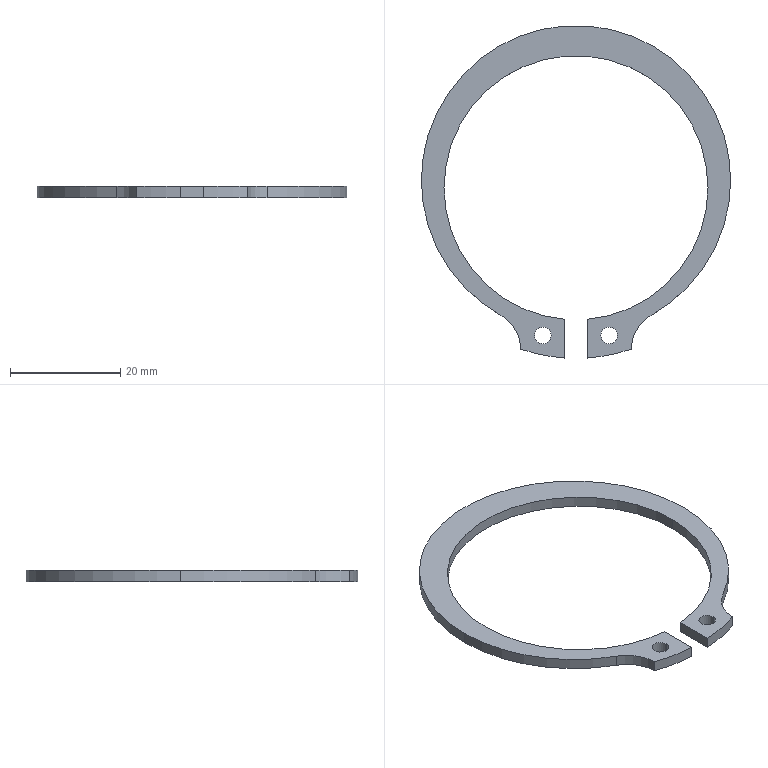Part | STEP file | circlips for shaft--type b gb_GB_CONNECTING_PIECE_RINGS_CSB 52 | 1 solid | 18 faces | box 56 x 60.185 x 2 mm | volume 1438 mm3 | cylinder 14 | plane 4 | commonest cylinder face diameters 3 x4 47.8 x3 56 x3 14 x2 61.76 x2
STEP:
#1=CARTESIAN_POINT('',(0.,0.,0.));
#2=DIRECTION('',(0.,0.,1.));
#3=DIRECTION('',(1.,0.,0.));
#4=AXIS2_PLACEMENT_3D('',#1,#2,#3);
#5=CARTESIAN_POINT('',(7.5,-28.105,-2.));
#6=VERTEX_POINT('',#5);
#7=CARTESIAN_POINT('',(7.5,-28.105,0.));
#8=VERTEX_POINT('',#7);
#9=CARTESIAN_POINT('',(7.5,-28.105,-2.));
#10=DIRECTION('',(0.,0.,1.));
#11=VECTOR('',#10,1.);
#12=LINE('',#9,#11);
#13=CARTESIAN_POINT('',(6.,-28.105,-2.));
#14=DIRECTION('',(0.,0.,1.));
#15=DIRECTION('',(1.,0.,0.));
#16=AXIS2_PLACEMENT_3D('',#13,#14,#15);
#17=CYLINDRICAL_SURFACE('',#16,1.5);
#18=CARTESIAN_POINT('',(6.283,0.));
#19=DIRECTION('',(0.,1.));
#20=VECTOR('',#19,1.);
#21=LINE('',#18,#20);
#22=(GEOMETRIC_REPRESENTATION_CONTEXT(2)PARAMETRIC_REPRESENTATION_CONTEXT()REPRESENTATION_CONTEXT('',''));
#23=DEFINITIONAL_REPRESENTATION('',(#21),#22);
#24=PCURVE('',#17,#23);
#25=CARTESIAN_POINT('',(6.,-28.105,-2.));
#26=DIRECTION('',(0.,0.,1.));
#27=DIRECTION('',(1.,0.,0.));
#28=AXIS2_PLACEMENT_3D('',#25,#26,#27);
#29=CYLINDRICAL_SURFACE('',#28,1.5);
#30=CARTESIAN_POINT('',(0.,0.));
#31=DIRECTION('',(0.,1.));
#32=VECTOR('',#31,1.);
#33=LINE('',#30,#32);
#34=(GEOMETRIC_REPRESENTATION_CONTEXT(2)PARAMETRIC_REPRESENTATION_CONTEXT()REPRESENTATION_CONTEXT('',''));
#35=DEFINITIONAL_REPRESENTATION('',(#33),#34);
#36=PCURVE('',#29,#35);
#37=SURFACE_CURVE('',#12,(#24,#36),.PCURVE_S1.);
#38=EDGE_CURVE('',#6,#8,#37,.T.);
#39=ORIENTED_EDGE('',*,*,#38,.T.);
#40=CARTESIAN_POINT('',(4.5,-28.105,0.));
#41=VERTEX_POINT('',#40);
#42=CARTESIAN_POINT('',(6.,-28.105,0.));
#43=DIRECTION('',(0.,0.,1.));
#44=DIRECTION('',(-1.,0.,0.));
#45=AXIS2_PLACEMENT_3D('',#42,#43,#44);
#46=CIRCLE('',#45,1.5);
#47=CARTESIAN_POINT('',(3.142,2.));
#48=DIRECTION('',(1.,0.));
#49=VECTOR('',#48,1.);
#50=LINE('',#47,#49);
#51=(GEOMETRIC_REPRESENTATION_CONTEXT(2)PARAMETRIC_REPRESENTATION_CONTEXT()REPRESENTATION_CONTEXT('',''));
#52=DEFINITIONAL_REPRESENTATION('',(#50),#51);
#53=PCURVE('',#17,#52);
#54=CARTESIAN_POINT('',(0.,0.,0.));
#55=DIRECTION('',(0.,0.,1.));
#56=DIRECTION('',(1.,0.,0.));
#57=AXIS2_PLACEMENT_3D('',#54,#55,#56);
#58=PLANE('',#57);
#59=CARTESIAN_POINT('',(6.,-28.105));
#60=DIRECTION('',(-1.,0.));
#61=AXIS2_PLACEMENT_2D('',#59,#60);
#62=CIRCLE('',#61,1.5);
#63=(GEOMETRIC_REPRESENTATION_CONTEXT(2)PARAMETRIC_REPRESENTATION_CONTEXT()REPRESENTATION_CONTEXT('',''));
#64=DEFINITIONAL_REPRESENTATION('',(#62),#63);
#65=PCURVE('',#58,#64);
#66=SURFACE_CURVE('',#46,(#53,#65),.PCURVE_S1.);
#67=EDGE_CURVE('',#41,#8,#66,.T.);
#68=ORIENTED_EDGE('',*,*,#67,.F.);
#69=CARTESIAN_POINT('',(4.5,-28.105,-2.));
#70=VERTEX_POINT('',#69);
#71=CARTESIAN_POINT('',(4.5,-28.105,-2.));
#72=DIRECTION('',(0.,0.,1.));
#73=VECTOR('',#72,1.);
#74=LINE('',#71,#73);
#75=CARTESIAN_POINT('',(3.142,0.));
#76=DIRECTION('',(0.,1.));
#77=VECTOR('',#76,1.);
#78=LINE('',#75,#77);
#79=(GEOMETRIC_REPRESENTATION_CONTEXT(2)PARAMETRIC_REPRESENTATION_CONTEXT()REPRESENTATION_CONTEXT('',''));
#80=DEFINITIONAL_REPRESENTATION('',(#78),#79);
#81=PCURVE('',#17,#80);
#82=CARTESIAN_POINT('',(3.142,0.));
#83=DIRECTION('',(0.,1.));
#84=VECTOR('',#83,1.);
#85=LINE('',#82,#84);
#86=(GEOMETRIC_REPRESENTATION_CONTEXT(2)PARAMETRIC_REPRESENTATION_CONTEXT()REPRESENTATION_CONTEXT('',''));
#87=DEFINITIONAL_REPRESENTATION('',(#85),#86);
#88=PCURVE('',#29,#87);
#89=SURFACE_CURVE('',#74,(#81,#88),.PCURVE_S1.);
#90=EDGE_CURVE('',#70,#41,#89,.T.);
#91=ORIENTED_EDGE('',*,*,#90,.F.);
#92=CARTESIAN_POINT('',(6.,-28.105,-2.));
#93=DIRECTION('',(0.,0.,1.));
#94=DIRECTION('',(-1.,0.,0.));
#95=AXIS2_PLACEMENT_3D('',#92,#93,#94);
#96=CIRCLE('',#95,1.5);
#97=CARTESIAN_POINT('',(3.142,0.));
#98=DIRECTION('',(1.,0.));
#99=VECTOR('',#98,1.);
#100=LINE('',#97,#99);
#101=(GEOMETRIC_REPRESENTATION_CONTEXT(2)PARAMETRIC_REPRESENTATION_CONTEXT()REPRESENTATION_CONTEXT('',''));
#102=DEFINITIONAL_REPRESENTATION('',(#100),#101);
#103=PCURVE('',#17,#102);
#104=CARTESIAN_POINT('',(0.,0.,-2.));
#105=DIRECTION('',(0.,0.,1.));
#106=DIRECTION('',(1.,0.,0.));
#107=AXIS2_PLACEMENT_3D('',#104,#105,#106);
#108=PLANE('',#107);
#109=CARTESIAN_POINT('',(6.,-28.105));
#110=DIRECTION('',(-1.,0.));
#111=AXIS2_PLACEMENT_2D('',#109,#110);
#112=CIRCLE('',#111,1.5);
#113=(GEOMETRIC_REPRESENTATION_CONTEXT(2)PARAMETRIC_REPRESENTATION_CONTEXT()REPRESENTATION_CONTEXT('',''));
#114=DEFINITIONAL_REPRESENTATION('',(#112),#113);
#115=PCURVE('',#108,#114);
#116=SURFACE_CURVE('',#96,(#103,#115),.PCURVE_S1.);
#117=EDGE_CURVE('',#70,#6,#116,.T.);
#118=ORIENTED_EDGE('',*,*,#117,.T.);
#119=EDGE_LOOP('',(#39,#68,#91,#118));
#120=FACE_BOUND('',#119,.F.);
#121=ADVANCED_FACE('',(#120),#17,.F.);
#122=CARTESIAN_POINT('',(-4.5,-28.105,-2.));
#123=VERTEX_POINT('',#122);
#124=CARTESIAN_POINT('',(-4.5,-28.105,0.));
#125=VERTEX_POINT('',#124);
#126=CARTESIAN_POINT('',(-4.5,-28.105,-2.));
#127=DIRECTION('',(0.,0.,1.));
#128=VECTOR('',#127,1.);
#129=LINE('',#126,#128);
#130=CARTESIAN_POINT('',(-6.,-28.105,-2.));
#131=DIRECTION('',(0.,0.,1.));
#132=DIRECTION('',(1.,0.,0.));
#133=AXIS2_PLACEMENT_3D('',#130,#131,#132);
#134=CYLINDRICAL_SURFACE('',#133,1.5);
#135=CARTESIAN_POINT('',(6.283,0.));
#136=DIRECTION('',(0.,1.));
#137=VECTOR('',#136,1.);
#138=LINE('',#135,#137);
#139=(GEOMETRIC_REPRESENTATION_CONTEXT(2)PARAMETRIC_REPRESENTATION_CONTEXT()REPRESENTATION_CONTEXT('',''));
#140=DEFINITIONAL_REPRESENTATION('',(#138),#139);
#141=PCURVE('',#134,#140);
#142=CARTESIAN_POINT('',(-6.,-28.105,-2.));
#143=DIRECTION('',(0.,0.,1.));
#144=DIRECTION('',(1.,0.,0.));
#145=AXIS2_PLACEMENT_3D('',#142,#143,#144);
#146=CYLINDRICAL_SURFACE('',#145,1.5);
#147=CARTESIAN_POINT('',(0.,0.));
#148=DIRECTION('',(0.,1.));
#149=VECTOR('',#148,1.);
#150=LINE('',#147,#149);
#151=(GEOMETRIC_REPRESENTATION_CONTEXT(2)PARAMETRIC_REPRESENTATION_CONTEXT()REPRESENTATION_CONTEXT('',''));
#152=DEFINITIONAL_REPRESENTATION('',(#150),#151);
#153=PCURVE('',#146,#152);
#154=SURFACE_CURVE('',#129,(#141,#153),.PCURVE_S1.);
#155=EDGE_CURVE('',#123,#125,#154,.T.);
#156=ORIENTED_EDGE('',*,*,#155,.T.);
#157=CARTESIAN_POINT('',(-7.5,-28.105,0.));
#158=VERTEX_POINT('',#157);
#159=CARTESIAN_POINT('',(-6.,-28.105,0.));
#160=DIRECTION('',(0.,0.,1.));
#161=DIRECTION('',(1.,0.,0.));
#162=AXIS2_PLACEMENT_3D('',#159,#160,#161);
#163=CIRCLE('',#162,1.5);
#164=CARTESIAN_POINT('',(0.,2.));
#165=DIRECTION('',(1.,0.));
#166=VECTOR('',#165,1.);
#167=LINE('',#164,#166);
#168=(GEOMETRIC_REPRESENTATION_CONTEXT(2)PARAMETRIC_REPRESENTATION_CONTEXT()REPRESENTATION_CONTEXT('',''));
#169=DEFINITIONAL_REPRESENTATION('',(#167),#168);
#170=PCURVE('',#134,#169);
#171=CARTESIAN_POINT('',(-6.,-28.105));
#172=DIRECTION('',(1.,0.));
#173=AXIS2_PLACEMENT_2D('',#171,#172);
#174=CIRCLE('',#173,1.5);
#175=(GEOMETRIC_REPRESENTATION_CONTEXT(2)PARAMETRIC_REPRESENTATION_CONTEXT()REPRESENTATION_CONTEXT('',''));
#176=DEFINITIONAL_REPRESENTATION('',(#174),#175);
#177=PCURVE('',#58,#176);
#178=SURFACE_CURVE('',#163,(#170,#177),.PCURVE_S1.);
#179=EDGE_CURVE('',#158,#125,#178,.T.);
#180=ORIENTED_EDGE('',*,*,#179,.F.);
#181=CARTESIAN_POINT('',(-7.5,-28.105,-2.));
#182=VERTEX_POINT('',#181);
#183=CARTESIAN_POINT('',(-7.5,-28.105,-2.));
#184=DIRECTION('',(0.,0.,1.));
#185=VECTOR('',#184,1.);
#186=LINE('',#183,#185);
#187=CARTESIAN_POINT('',(3.142,0.));
#188=DIRECTION('',(0.,1.));
#189=VECTOR('',#188,1.);
#190=LINE('',#187,#189);
#191=(GEOMETRIC_REPRESENTATION_CONTEXT(2)PARAMETRIC_REPRESENTATION_CONTEXT()REPRESENTATION_CONTEXT('',''));
#192=DEFINITIONAL_REPRESENTATION('',(#190),#191);
#193=PCURVE('',#134,#192);
#194=CARTESIAN_POINT('',(3.142,0.));
#195=DIRECTION('',(0.,1.));
#196=VECTOR('',#195,1.);
#197=LINE('',#194,#196);
#198=(GEOMETRIC_REPRESENTATION_CONTEXT(2)PARAMETRIC_REPRESENTATION_CONTEXT()REPRESENTATION_CONTEXT('',''));
#199=DEFINITIONAL_REPRESENTATION('',(#197),#198);
#200=PCURVE('',#146,#199);
#201=SURFACE_CURVE('',#186,(#193,#200),.PCURVE_S1.);
#202=EDGE_CURVE('',#182,#158,#201,.T.);
#203=ORIENTED_EDGE('',*,*,#202,.F.);
#204=CARTESIAN_POINT('',(-6.,-28.105,-2.));
#205=DIRECTION('',(0.,0.,1.));
#206=DIRECTION('',(1.,0.,0.));
#207=AXIS2_PLACEMENT_3D('',#204,#205,#206);
#208=CIRCLE('',#207,1.5);
#209=CARTESIAN_POINT('',(0.,0.));
#210=DIRECTION('',(1.,0.));
#211=VECTOR('',#210,1.);
#212=LINE('',#209,#211);
#213=(GEOMETRIC_REPRESENTATION_CONTEXT(2)PARAMETRIC_REPRESENTATION_CONTEXT()REPRESENTATION_CONTEXT('',''));
#214=DEFINITIONAL_REPRESENTATION('',(#212),#213);
#215=PCURVE('',#134,#214);
#216=CARTESIAN_POINT('',(-6.,-28.105));
#217=DIRECTION('',(1.,0.));
#218=AXIS2_PLACEMENT_2D('',#216,#217);
#219=CIRCLE('',#218,1.5);
#220=(GEOMETRIC_REPRESENTATION_CONTEXT(2)PARAMETRIC_REPRESENTATION_CONTEXT()REPRESENTATION_CONTEXT('',''));
#221=DEFINITIONAL_REPRESENTATION('',(#219),#220);
#222=PCURVE('',#108,#221);
#223=SURFACE_CURVE('',#208,(#215,#222),.PCURVE_S1.);
#224=EDGE_CURVE('',#182,#123,#223,.T.);
#225=ORIENTED_EDGE('',*,*,#224,.T.);
#226=EDGE_LOOP('',(#156,#180,#203,#225));
#227=FACE_BOUND('',#226,.F.);
#228=ADVANCED_FACE('',(#227),#134,.F.);
#229=CARTESIAN_POINT('',(-2.,-25.186,-2.));
#230=VERTEX_POINT('',#229);
#231=CARTESIAN_POINT('',(-2.,-25.186,0.));
#232=VERTEX_POINT('',#231);
#233=CARTESIAN_POINT('',(-2.,-25.186,-2.));
#234=DIRECTION('',(0.,0.,1.));
#235=VECTOR('',#234,1.);
#236=LINE('',#233,#235);
#237=CARTESIAN_POINT('',(0.,-1.37,-2.));
#238=DIRECTION('',(0.,0.,1.));
#239=DIRECTION('',(1.,0.,0.));
#240=AXIS2_PLACEMENT_3D('',#237,#238,#239);
#241=CYLINDRICAL_SURFACE('',#240,23.9);
#242=CARTESIAN_POINT('',(4.629,0.));
#243=DIRECTION('',(0.,1.));
#244=VECTOR('',#243,1.);
#245=LINE('',#242,#244);
#246=(GEOMETRIC_REPRESENTATION_CONTEXT(2)PARAMETRIC_REPRESENTATION_CONTEXT()REPRESENTATION_CONTEXT('',''));
#247=DEFINITIONAL_REPRESENTATION('',(#245),#246);
#248=PCURVE('',#241,#247);
#249=CARTESIAN_POINT('',(-2.,-32.185,-2.));
#250=DIRECTION('',(1.,0.,0.));
#251=DIRECTION('',(0.,1.,0.));
#252=AXIS2_PLACEMENT_3D('',#249,#250,#251);
#253=PLANE('',#252);
#254=CARTESIAN_POINT('',(6.999,0.));
#255=DIRECTION('',(0.,1.));
#256=VECTOR('',#255,1.);
#257=LINE('',#254,#256);
#258=(GEOMETRIC_REPRESENTATION_CONTEXT(2)PARAMETRIC_REPRESENTATION_CONTEXT()REPRESENTATION_CONTEXT('',''));
#259=DEFINITIONAL_REPRESENTATION('',(#257),#258);
#260=PCURVE('',#253,#259);
#261=SURFACE_CURVE('',#236,(#248,#260),.PCURVE_S1.);
#262=EDGE_CURVE('',#230,#232,#261,.T.);
#263=ORIENTED_EDGE('',*,*,#262,.T.);
#264=CARTESIAN_POINT('',(-23.9,-1.37,0.));
#265=VERTEX_POINT('',#264);
#266=CARTESIAN_POINT('',(0.,-1.37,0.));
#267=DIRECTION('',(0.,0.,-1.));
#268=DIRECTION('',(1.,0.,0.));
#269=AXIS2_PLACEMENT_3D('',#266,#267,#268);
#270=CIRCLE('',#269,23.9);
#271=CARTESIAN_POINT('',(6.283,2.));
#272=DIRECTION('',(-1.,0.));
#273=VECTOR('',#272,1.);
#274=LINE('',#271,#273);
#275=(GEOMETRIC_REPRESENTATION_CONTEXT(2)PARAMETRIC_REPRESENTATION_CONTEXT()REPRESENTATION_CONTEXT('',''));
#276=DEFINITIONAL_REPRESENTATION('',(#274),#275);
#277=PCURVE('',#241,#276);
#278=CARTESIAN_POINT('',(23.9,-1.37));
#279=CARTESIAN_POINT('',(23.9,-42.766));
#280=CARTESIAN_POINT('',(-11.95,-22.068));
#281=CARTESIAN_POINT('',(-47.8,-1.37));
#282=CARTESIAN_POINT('',(-11.95,19.328));
#283=CARTESIAN_POINT('',(23.9,40.026));
#284=CARTESIAN_POINT('',(23.9,-1.37));
#285=(BOUNDED_CURVE()B_SPLINE_CURVE(2,(#278,#279,#280,#281,#282,#283,#284),.UNSPECIFIED.,.T.,.F.)B_SPLINE_CURVE_WITH_KNOTS((1,2,2,2,2,1),(-2.094,0.,2.094,4.189,6.283,8.378),.UNSPECIFIED.)CURVE()GEOMETRIC_REPRESENTATION_ITEM()RATIONAL_B_SPLINE_CURVE((1.,0.5,1.,0.5,1.,0.5,1.))REPRESENTATION_ITEM(''));
#286=(GEOMETRIC_REPRESENTATION_CONTEXT(2)PARAMETRIC_REPRESENTATION_CONTEXT()REPRESENTATION_CONTEXT('',''));
#287=DEFINITIONAL_REPRESENTATION('',(#285),#286);
#288=PCURVE('',#58,#287);
#289=SURFACE_CURVE('',#270,(#277,#288),.PCURVE_S1.);
#290=EDGE_CURVE('',#232,#265,#289,.T.);
#291=ORIENTED_EDGE('',*,*,#290,.T.);
#292=CARTESIAN_POINT('',(-23.9,-1.37,-2.));
#293=VERTEX_POINT('',#292);
#294=CARTESIAN_POINT('',(-23.9,-1.37,-2.));
#295=DIRECTION('',(0.,0.,1.));
#296=VECTOR('',#295,1.);
#297=LINE('',#294,#296);
#298=CARTESIAN_POINT('',(3.142,0.));
#299=DIRECTION('',(0.,1.));
#300=VECTOR('',#299,1.);
#301=LINE('',#298,#300);
#302=(GEOMETRIC_REPRESENTATION_CONTEXT(2)PARAMETRIC_REPRESENTATION_CONTEXT()REPRESENTATION_CONTEXT('',''));
#303=DEFINITIONAL_REPRESENTATION('',(#301),#302);
#304=PCURVE('',#241,#303);
#305=CARTESIAN_POINT('',(0.,-1.37,-2.));
#306=DIRECTION('',(0.,0.,1.));
#307=DIRECTION('',(1.,0.,0.));
#308=AXIS2_PLACEMENT_3D('',#305,#306,#307);
#309=CYLINDRICAL_SURFACE('',#308,23.9);
#310=CARTESIAN_POINT('',(3.142,0.));
#311=DIRECTION('',(0.,1.));
#312=VECTOR('',#311,1.);
#313=LINE('',#310,#312);
#314=(GEOMETRIC_REPRESENTATION_CONTEXT(2)PARAMETRIC_REPRESENTATION_CONTEXT()REPRESENTATION_CONTEXT('',''));
#315=DEFINITIONAL_REPRESENTATION('',(#313),#314);
#316=PCURVE('',#309,#315);
#317=SURFACE_CURVE('',#297,(#304,#316),.PCURVE_S1.);
#318=EDGE_CURVE('',#293,#265,#317,.T.);
#319=ORIENTED_EDGE('',*,*,#318,.F.);
#320=CARTESIAN_POINT('',(0.,-1.37,-2.));
#321=DIRECTION('',(0.,0.,-1.));
#322=DIRECTION('',(1.,0.,0.));
#323=AXIS2_PLACEMENT_3D('',#320,#321,#322);
#324=CIRCLE('',#323,23.9);
#325=CARTESIAN_POINT('',(6.283,0.));
#326=DIRECTION('',(-1.,0.));
#327=VECTOR('',#326,1.);
#328=LINE('',#325,#327);
#329=(GEOMETRIC_REPRESENTATION_CONTEXT(2)PARAMETRIC_REPRESENTATION_CONTEXT()REPRESENTATION_CONTEXT('',''));
#330=DEFINITIONAL_REPRESENTATION('',(#328),#329);
#331=PCURVE('',#241,#330);
#332=CARTESIAN_POINT('',(23.9,-1.37));
#333=CARTESIAN_POINT('',(23.9,-42.766));
#334=CARTESIAN_POINT('',(-11.95,-22.068));
#335=CARTESIAN_POINT('',(-47.8,-1.37));
#336=CARTESIAN_POINT('',(-11.95,19.328));
#337=CARTESIAN_POINT('',(23.9,40.026));
#338=CARTESIAN_POINT('',(23.9,-1.37));
#339=(BOUNDED_CURVE()B_SPLINE_CURVE(2,(#332,#333,#334,#335,#336,#337,#338),.UNSPECIFIED.,.T.,.F.)B_SPLINE_CURVE_WITH_KNOTS((1,2,2,2,2,1),(-2.094,0.,2.094,4.189,6.283,8.378),.UNSPECIFIED.)CURVE()GEOMETRIC_REPRESENTATION_ITEM()RATIONAL_B_SPLINE_CURVE((1.,0.5,1.,0.5,1.,0.5,1.))REPRESENTATION_ITEM(''));
#340=(GEOMETRIC_REPRESENTATION_CONTEXT(2)PARAMETRIC_REPRESENTATION_CONTEXT()REPRESENTATION_CONTEXT('',''));
#341=DEFINITIONAL_REPRESENTATION('',(#339),#340);
#342=PCURVE('',#108,#341);
#343=SURFACE_CURVE('',#324,(#331,#342),.PCURVE_S1.);
#344=EDGE_CURVE('',#230,#293,#343,.T.);
#345=ORIENTED_EDGE('',*,*,#344,.F.);
#346=EDGE_LOOP('',(#263,#291,#319,#345));
#347=FACE_BOUND('',#346,.F.);
#348=ADVANCED_FACE('',(#347),#241,.F.);
#349=CARTESIAN_POINT('',(23.9,-1.37,0.));
#350=VERTEX_POINT('',#349);
#351=CARTESIAN_POINT('',(0.,-1.37,0.));
#352=DIRECTION('',(0.,0.,-1.));
#353=DIRECTION('',(1.,0.,0.));
#354=AXIS2_PLACEMENT_3D('',#351,#352,#353);
#355=CIRCLE('',#354,23.9);
#356=CARTESIAN_POINT('',(6.283,2.));
#357=DIRECTION('',(-1.,0.));
#358=VECTOR('',#357,1.);
#359=LINE('',#356,#358);
#360=(GEOMETRIC_REPRESENTATION_CONTEXT(2)PARAMETRIC_REPRESENTATION_CONTEXT()REPRESENTATION_CONTEXT('',''));
#361=DEFINITIONAL_REPRESENTATION('',(#359),#360);
#362=PCURVE('',#309,#361);
#363=CARTESIAN_POINT('',(23.9,-1.37));
#364=CARTESIAN_POINT('',(23.9,-42.766));
#365=CARTESIAN_POINT('',(-11.95,-22.068));
#366=CARTESIAN_POINT('',(-47.8,-1.37));
#367=CARTESIAN_POINT('',(-11.95,19.328));
#368=CARTESIAN_POINT('',(23.9,40.026));
#369=CARTESIAN_POINT('',(23.9,-1.37));
#370=(BOUNDED_CURVE()B_SPLINE_CURVE(2,(#363,#364,#365,#366,#367,#368,#369),.UNSPECIFIED.,.T.,.F.)B_SPLINE_CURVE_WITH_KNOTS((1,2,2,2,2,1),(-2.094,0.,2.094,4.189,6.283,8.378),.UNSPECIFIED.)CURVE()GEOMETRIC_REPRESENTATION_ITEM()RATIONAL_B_SPLINE_CURVE((1.,0.5,1.,0.5,1.,0.5,1.))REPRESENTATION_ITEM(''));
#371=(GEOMETRIC_REPRESENTATION_CONTEXT(2)PARAMETRIC_REPRESENTATION_CONTEXT()REPRESENTATION_CONTEXT('',''));
#372=DEFINITIONAL_REPRESENTATION('',(#370),#371);
#373=PCURVE('',#58,#372);
#374=SURFACE_CURVE('',#355,(#362,#373),.PCURVE_S1.);
#375=EDGE_CURVE('',#265,#350,#374,.T.);
#376=ORIENTED_EDGE('',*,*,#375,.T.);
#377=CARTESIAN_POINT('',(23.9,-1.37,-2.));
#378=VERTEX_POINT('',#377);
#379=CARTESIAN_POINT('',(23.9,-1.37,-2.));
#380=DIRECTION('',(0.,0.,1.));
#381=VECTOR('',#380,1.);
#382=LINE('',#379,#381);
#383=CARTESIAN_POINT('',(0.,0.));
#384=DIRECTION('',(0.,1.));
#385=VECTOR('',#384,1.);
#386=LINE('',#383,#385);
#387=(GEOMETRIC_REPRESENTATION_CONTEXT(2)PARAMETRIC_REPRESENTATION_CONTEXT()REPRESENTATION_CONTEXT('',''));
#388=DEFINITIONAL_REPRESENTATION('',(#386),#387);
#389=PCURVE('',#309,#388);
#390=CARTESIAN_POINT('',(0.,-1.37,-2.));
#391=DIRECTION('',(0.,0.,1.));
#392=DIRECTION('',(1.,0.,0.));
#393=AXIS2_PLACEMENT_3D('',#390,#391,#392);
#394=CYLINDRICAL_SURFACE('',#393,23.9);
#395=CARTESIAN_POINT('',(6.283,0.));
#396=DIRECTION('',(0.,1.));
#397=VECTOR('',#396,1.);
#398=LINE('',#395,#397);
#399=(GEOMETRIC_REPRESENTATION_CONTEXT(2)PARAMETRIC_REPRESENTATION_CONTEXT()REPRESENTATION_CONTEXT('',''));
#400=DEFINITIONAL_REPRESENTATION('',(#398),#399);
#401=PCURVE('',#394,#400);
#402=SURFACE_CURVE('',#382,(#389,#401),.PCURVE_S1.);
#403=EDGE_CURVE('',#378,#350,#402,.T.);
#404=ORIENTED_EDGE('',*,*,#403,.F.);
#405=CARTESIAN_POINT('',(0.,-1.37,-2.));
#406=DIRECTION('',(0.,0.,-1.));
#407=DIRECTION('',(1.,0.,0.));
#408=AXIS2_PLACEMENT_3D('',#405,#406,#407);
#409=CIRCLE('',#408,23.9);
#410=CARTESIAN_POINT('',(6.283,0.));
#411=DIRECTION('',(-1.,0.));
#412=VECTOR('',#411,1.);
#413=LINE('',#410,#412);
#414=(GEOMETRIC_REPRESENTATION_CONTEXT(2)PARAMETRIC_REPRESENTATION_CONTEXT()REPRESENTATION_CONTEXT('',''));
#415=DEFINITIONAL_REPRESENTATION('',(#413),#414);
#416=PCURVE('',#309,#415);
#417=CARTESIAN_POINT('',(23.9,-1.37));
#418=CARTESIAN_POINT('',(23.9,-42.766));
#419=CARTESIAN_POINT('',(-11.95,-22.068));
#420=CARTESIAN_POINT('',(-47.8,-1.37));
#421=CARTESIAN_POINT('',(-11.95,19.328));
#422=CARTESIAN_POINT('',(23.9,40.026));
#423=CARTESIAN_POINT('',(23.9,-1.37));
#424=(BOUNDED_CURVE()B_SPLINE_CURVE(2,(#417,#418,#419,#420,#421,#422,#423),.UNSPECIFIED.,.T.,.F.)B_SPLINE_CURVE_WITH_KNOTS((1,2,2,2,2,1),(-2.094,0.,2.094,4.189,6.283,8.378),.UNSPECIFIED.)CURVE()GEOMETRIC_REPRESENTATION_ITEM()RATIONAL_B_SPLINE_CURVE((1.,0.5,1.,0.5,1.,0.5,1.))REPRESENTATION_ITEM(''));
#425=(GEOMETRIC_REPRESENTATION_CONTEXT(2)PARAMETRIC_REPRESENTATION_CONTEXT()REPRESENTATION_CONTEXT('',''));
#426=DEFINITIONAL_REPRESENTATION('',(#424),#425);
#427=PCURVE('',#108,#426);
#428=SURFACE_CURVE('',#409,(#416,#427),.PCURVE_S1.);
#429=EDGE_CURVE('',#293,#378,#428,.T.);
#430=ORIENTED_EDGE('',*,*,#429,.F.);
#431=ORIENTED_EDGE('',*,*,#318,.T.);
#432=EDGE_LOOP('',(#376,#404,#430,#431));
#433=FACE_BOUND('',#432,.F.);
#434=ADVANCED_FACE('',(#433),#309,.F.);
#435=CARTESIAN_POINT('',(28.,0.,-2.));
#436=VERTEX_POINT('',#435);
#437=CARTESIAN_POINT('',(-28.,0.,-2.));
#438=VERTEX_POINT('',#437);
#439=CARTESIAN_POINT('',(0.,0.,-2.));
#440=DIRECTION('',(0.,0.,1.));
#441=DIRECTION('',(1.,0.,0.));
#442=AXIS2_PLACEMENT_3D('',#439,#440,#441);
#443=CIRCLE('',#442,28.);
#444=CARTESIAN_POINT('',(0.,0.,-2.));
#445=DIRECTION('',(0.,0.,1.));
#446=DIRECTION('',(1.,0.,0.));
#447=AXIS2_PLACEMENT_3D('',#444,#445,#446);
#448=CYLINDRICAL_SURFACE('',#447,28.);
#449=CARTESIAN_POINT('',(0.,0.));
#450=DIRECTION('',(1.,0.));
#451=VECTOR('',#450,1.);
#452=LINE('',#449,#451);
#453=(GEOMETRIC_REPRESENTATION_CONTEXT(2)PARAMETRIC_REPRESENTATION_CONTEXT()REPRESENTATION_CONTEXT('',''));
#454=DEFINITIONAL_REPRESENTATION('',(#452),#453);
#455=PCURVE('',#448,#454);
#456=CARTESIAN_POINT('',(0.,0.));
#457=DIRECTION('',(1.,0.));
#458=AXIS2_PLACEMENT_2D('',#456,#457);
#459=CIRCLE('',#458,28.);
#460=(GEOMETRIC_REPRESENTATION_CONTEXT(2)PARAMETRIC_REPRESENTATION_CONTEXT()REPRESENTATION_CONTEXT('',''));
#461=DEFINITIONAL_REPRESENTATION('',(#459),#460);
#462=PCURVE('',#108,#461);
#463=SURFACE_CURVE('',#443,(#455,#462),.PCURVE_S1.);
#464=EDGE_CURVE('',#436,#438,#463,.T.);
#465=ORIENTED_EDGE('',*,*,#464,.T.);
#466=CARTESIAN_POINT('',(-28.,0.,0.));
#467=VERTEX_POINT('',#466);
#468=CARTESIAN_POINT('',(-28.,0.,-2.));
#469=DIRECTION('',(0.,0.,1.));
#470=VECTOR('',#469,1.);
#471=LINE('',#468,#470);
#472=CARTESIAN_POINT('',(3.142,0.));
#473=DIRECTION('',(0.,1.));
#474=VECTOR('',#473,1.);
#475=LINE('',#472,#474);
#476=(GEOMETRIC_REPRESENTATION_CONTEXT(2)PARAMETRIC_REPRESENTATION_CONTEXT()REPRESENTATION_CONTEXT('',''));
#477=DEFINITIONAL_REPRESENTATION('',(#475),#476);
#478=PCURVE('',#448,#477);
#479=CARTESIAN_POINT('',(0.,0.,-2.));
#480=DIRECTION('',(0.,0.,1.));
#481=DIRECTION('',(1.,0.,0.));
#482=AXIS2_PLACEMENT_3D('',#479,#480,#481);
#483=CYLINDRICAL_SURFACE('',#482,28.);
#484=CARTESIAN_POINT('',(3.142,0.));
#485=DIRECTION('',(0.,1.));
#486=VECTOR('',#485,1.);
#487=LINE('',#484,#486);
#488=(GEOMETRIC_REPRESENTATION_CONTEXT(2)PARAMETRIC_REPRESENTATION_CONTEXT()REPRESENTATION_CONTEXT('',''));
#489=DEFINITIONAL_REPRESENTATION('',(#487),#488);
#490=PCURVE('',#483,#489);
#491=SURFACE_CURVE('',#471,(#478,#490),.PCURVE_S1.);
#492=EDGE_CURVE('',#438,#467,#491,.T.);
#493=ORIENTED_EDGE('',*,*,#492,.T.);
#494=CARTESIAN_POINT('',(28.,0.,0.));
#495=VERTEX_POINT('',#494);
#496=CARTESIAN_POINT('',(0.,0.,0.));
#497=DIRECTION('',(0.,0.,1.));
#498=DIRECTION('',(1.,0.,0.));
#499=AXIS2_PLACEMENT_3D('',#496,#497,#498);
#500=CIRCLE('',#499,28.);
#501=CARTESIAN_POINT('',(0.,2.));
#502=DIRECTION('',(1.,0.));
#503=VECTOR('',#502,1.);
#504=LINE('',#501,#503);
#505=(GEOMETRIC_REPRESENTATION_CONTEXT(2)PARAMETRIC_REPRESENTATION_CONTEXT()REPRESENTATION_CONTEXT('',''));
#506=DEFINITIONAL_REPRESENTATION('',(#504),#505);
#507=PCURVE('',#448,#506);
#508=CARTESIAN_POINT('',(0.,0.));
#509=DIRECTION('',(1.,0.));
#510=AXIS2_PLACEMENT_2D('',#508,#509);
#511=CIRCLE('',#510,28.);
#512=(GEOMETRIC_REPRESENTATION_CONTEXT(2)PARAMETRIC_REPRESENTATION_CONTEXT()REPRESENTATION_CONTEXT('',''));
#513=DEFINITIONAL_REPRESENTATION('',(#511),#512);
#514=PCURVE('',#58,#513);
#515=SURFACE_CURVE('',#500,(#507,#514),.PCURVE_S1.);
#516=EDGE_CURVE('',#495,#467,#515,.T.);
#517=ORIENTED_EDGE('',*,*,#516,.F.);
#518=CARTESIAN_POINT('',(28.,0.,-2.));
#519=DIRECTION('',(0.,0.,1.));
#520=VECTOR('',#519,1.);
#521=LINE('',#518,#520);
#522=CARTESIAN_POINT('',(0.,0.));
#523=DIRECTION('',(0.,1.));
#524=VECTOR('',#523,1.);
#525=LINE('',#522,#524);
#526=(GEOMETRIC_REPRESENTATION_CONTEXT(2)PARAMETRIC_REPRESENTATION_CONTEXT()REPRESENTATION_CONTEXT('',''));
#527=DEFINITIONAL_REPRESENTATION('',(#525),#526);
#528=PCURVE('',#448,#527);
#529=CARTESIAN_POINT('',(0.,0.,-2.));
#530=DIRECTION('',(0.,0.,1.));
#531=DIRECTION('',(1.,0.,0.));
#532=AXIS2_PLACEMENT_3D('',#529,#530,#531);
#533=CYLINDRICAL_SURFACE('',#532,28.);
#534=CARTESIAN_POINT('',(6.283,0.));
#535=DIRECTION('',(0.,1.));
#536=VECTOR('',#535,1.);
#537=LINE('',#534,#536);
#538=(GEOMETRIC_REPRESENTATION_CONTEXT(2)PARAMETRIC_REPRESENTATION_CONTEXT()REPRESENTATION_CONTEXT('',''));
#539=DEFINITIONAL_REPRESENTATION('',(#537),#538);
#540=PCURVE('',#533,#539);
#541=SURFACE_CURVE('',#521,(#528,#540),.PCURVE_S1.);
#542=EDGE_CURVE('',#436,#495,#541,.T.);
#543=ORIENTED_EDGE('',*,*,#542,.F.);
#544=EDGE_LOOP('',(#465,#493,#517,#543));
#545=FACE_BOUND('',#544,.T.);
#546=ADVANCED_FACE('',(#545),#448,.T.);
#547=CARTESIAN_POINT('',(13.6,-24.475,-2.));
#548=VERTEX_POINT('',#547);
#549=CARTESIAN_POINT('',(0.,0.,-2.));
#550=DIRECTION('',(0.,0.,1.));
#551=DIRECTION('',(1.,0.,0.));
#552=AXIS2_PLACEMENT_3D('',#549,#550,#551);
#553=CIRCLE('',#552,28.);
#554=CARTESIAN_POINT('',(0.,0.));
#555=DIRECTION('',(1.,0.));
#556=VECTOR('',#555,1.);
#557=LINE('',#554,#556);
#558=(GEOMETRIC_REPRESENTATION_CONTEXT(2)PARAMETRIC_REPRESENTATION_CONTEXT()REPRESENTATION_CONTEXT('',''));
#559=DEFINITIONAL_REPRESENTATION('',(#557),#558);
#560=PCURVE('',#533,#559);
#561=CARTESIAN_POINT('',(0.,0.));
#562=DIRECTION('',(1.,0.));
#563=AXIS2_PLACEMENT_2D('',#561,#562);
#564=CIRCLE('',#563,28.);
#565=(GEOMETRIC_REPRESENTATION_CONTEXT(2)PARAMETRIC_REPRESENTATION_CONTEXT()REPRESENTATION_CONTEXT('',''));
#566=DEFINITIONAL_REPRESENTATION('',(#564),#565);
#567=PCURVE('',#108,#566);
#568=SURFACE_CURVE('',#553,(#560,#567),.PCURVE_S1.);
#569=EDGE_CURVE('',#548,#436,#568,.T.);
#570=ORIENTED_EDGE('',*,*,#569,.T.);
#571=ORIENTED_EDGE('',*,*,#542,.T.);
#572=CARTESIAN_POINT('',(13.6,-24.475,0.));
#573=VERTEX_POINT('',#572);
#574=CARTESIAN_POINT('',(0.,0.,0.));
#575=DIRECTION('',(0.,0.,1.));
#576=DIRECTION('',(1.,0.,0.));
#577=AXIS2_PLACEMENT_3D('',#574,#575,#576);
#578=CIRCLE('',#577,28.);
#579=CARTESIAN_POINT('',(0.,2.));
#580=DIRECTION('',(1.,0.));
#581=VECTOR('',#580,1.);
#582=LINE('',#579,#581);
#583=(GEOMETRIC_REPRESENTATION_CONTEXT(2)PARAMETRIC_REPRESENTATION_CONTEXT()REPRESENTATION_CONTEXT('',''));
#584=DEFINITIONAL_REPRESENTATION('',(#582),#583);
#585=PCURVE('',#533,#584);
#586=CARTESIAN_POINT('',(0.,0.));
#587=DIRECTION('',(1.,0.));
#588=AXIS2_PLACEMENT_2D('',#586,#587);
#589=CIRCLE('',#588,28.);
#590=(GEOMETRIC_REPRESENTATION_CONTEXT(2)PARAMETRIC_REPRESENTATION_CONTEXT()REPRESENTATION_CONTEXT('',''));
#591=DEFINITIONAL_REPRESENTATION('',(#589),#590);
#592=PCURVE('',#58,#591);
#593=SURFACE_CURVE('',#578,(#585,#592),.PCURVE_S1.);
#594=EDGE_CURVE('',#573,#495,#593,.T.);
#595=ORIENTED_EDGE('',*,*,#594,.F.);
#596=CARTESIAN_POINT('',(13.6,-24.475,-2.));
#597=DIRECTION('',(0.,0.,-1.));
#598=VECTOR('',#597,1.);
#599=LINE('',#596,#598);
#600=CARTESIAN_POINT('',(5.22,0.));
#601=DIRECTION('',(0.,-1.));
#602=VECTOR('',#601,1.);
#603=LINE('',#600,#602);
#604=(GEOMETRIC_REPRESENTATION_CONTEXT(2)PARAMETRIC_REPRESENTATION_CONTEXT()REPRESENTATION_CONTEXT('',''));
#605=DEFINITIONAL_REPRESENTATION('',(#603),#604);
#606=PCURVE('',#533,#605);
#607=CARTESIAN_POINT('',(17.,-30.594,-2.));
#608=DIRECTION('',(0.,0.,-1.));
#609=DIRECTION('',(-1.,0.,0.));
#610=AXIS2_PLACEMENT_3D('',#607,#608,#609);
#611=CYLINDRICAL_SURFACE('',#610,7.);
#612=CARTESIAN_POINT('',(1.064,0.));
#613=DIRECTION('',(0.,1.));
#614=VECTOR('',#613,1.);
#615=LINE('',#612,#614);
#616=(GEOMETRIC_REPRESENTATION_CONTEXT(2)PARAMETRIC_REPRESENTATION_CONTEXT()REPRESENTATION_CONTEXT('',''));
#617=DEFINITIONAL_REPRESENTATION('',(#615),#616);
#618=PCURVE('',#611,#617);
#619=SURFACE_CURVE('',#599,(#606,#618),.PCURVE_S1.);
#620=EDGE_CURVE('',#573,#548,#619,.T.);
#621=ORIENTED_EDGE('',*,*,#620,.T.);
#622=EDGE_LOOP('',(#570,#571,#595,#621));
#623=FACE_BOUND('',#622,.T.);
#624=ADVANCED_FACE('',(#623),#533,.T.);
#625=ORIENTED_EDGE('',*,*,#492,.F.);
#626=CARTESIAN_POINT('',(-13.6,-24.475,-2.));
#627=VERTEX_POINT('',#626);
#628=CARTESIAN_POINT('',(0.,0.,-2.));
#629=DIRECTION('',(0.,0.,1.));
#630=DIRECTION('',(1.,0.,0.));
#631=AXIS2_PLACEMENT_3D('',#628,#629,#630);
#632=CIRCLE('',#631,28.);
#633=CARTESIAN_POINT('',(0.,0.));
#634=DIRECTION('',(1.,0.));
#635=VECTOR('',#634,1.);
#636=LINE('',#633,#635);
#637=(GEOMETRIC_REPRESENTATION_CONTEXT(2)PARAMETRIC_REPRESENTATION_CONTEXT()REPRESENTATION_CONTEXT('',''));
#638=DEFINITIONAL_REPRESENTATION('',(#636),#637);
#639=PCURVE('',#483,#638);
#640=CARTESIAN_POINT('',(0.,0.));
#641=DIRECTION('',(1.,0.));
#642=AXIS2_PLACEMENT_2D('',#640,#641);
#643=CIRCLE('',#642,28.);
#644=(GEOMETRIC_REPRESENTATION_CONTEXT(2)PARAMETRIC_REPRESENTATION_CONTEXT()REPRESENTATION_CONTEXT('',''));
#645=DEFINITIONAL_REPRESENTATION('',(#643),#644);
#646=PCURVE('',#108,#645);
#647=SURFACE_CURVE('',#632,(#639,#646),.PCURVE_S1.);
#648=EDGE_CURVE('',#438,#627,#647,.T.);
#649=ORIENTED_EDGE('',*,*,#648,.T.);
#650=CARTESIAN_POINT('',(-13.6,-24.475,0.));
#651=VERTEX_POINT('',#650);
#652=CARTESIAN_POINT('',(-13.6,-24.475,-2.));
#653=DIRECTION('',(0.,0.,1.));
#654=VECTOR('',#653,1.);
#655=LINE('',#652,#654);
#656=CARTESIAN_POINT('',(4.205,0.));
#657=DIRECTION('',(0.,1.));
#658=VECTOR('',#657,1.);
#659=LINE('',#656,#658);
#660=(GEOMETRIC_REPRESENTATION_CONTEXT(2)PARAMETRIC_REPRESENTATION_CONTEXT()REPRESENTATION_CONTEXT('',''));
#661=DEFINITIONAL_REPRESENTATION('',(#659),#660);
#662=PCURVE('',#483,#661);
#663=CARTESIAN_POINT('',(-17.,-30.594,-2.));
#664=DIRECTION('',(0.,0.,-1.));
#665=DIRECTION('',(-1.,0.,0.));
#666=AXIS2_PLACEMENT_3D('',#663,#664,#665);
#667=CYLINDRICAL_SURFACE('',#666,7.);
#668=CARTESIAN_POINT('',(2.078,0.));
#669=DIRECTION('',(0.,-1.));
#670=VECTOR('',#669,1.);
#671=LINE('',#668,#670);
#672=(GEOMETRIC_REPRESENTATION_CONTEXT(2)PARAMETRIC_REPRESENTATION_CONTEXT()REPRESENTATION_CONTEXT('',''));
#673=DEFINITIONAL_REPRESENTATION('',(#671),#672);
#674=PCURVE('',#667,#673);
#675=SURFACE_CURVE('',#655,(#662,#674),.PCURVE_S1.);
#676=EDGE_CURVE('',#627,#651,#675,.T.);
#677=ORIENTED_EDGE('',*,*,#676,.T.);
#678=CARTESIAN_POINT('',(0.,0.,0.));
#679=DIRECTION('',(0.,0.,1.));
#680=DIRECTION('',(1.,0.,0.));
#681=AXIS2_PLACEMENT_3D('',#678,#679,#680);
#682=CIRCLE('',#681,28.);
#683=CARTESIAN_POINT('',(0.,2.));
#684=DIRECTION('',(1.,0.));
#685=VECTOR('',#684,1.);
#686=LINE('',#683,#685);
#687=(GEOMETRIC_REPRESENTATION_CONTEXT(2)PARAMETRIC_REPRESENTATION_CONTEXT()REPRESENTATION_CONTEXT('',''));
#688=DEFINITIONAL_REPRESENTATION('',(#686),#687);
#689=PCURVE('',#483,#688);
#690=CARTESIAN_POINT('',(0.,0.));
#691=DIRECTION('',(1.,0.));
#692=AXIS2_PLACEMENT_2D('',#690,#691);
#693=CIRCLE('',#692,28.);
#694=(GEOMETRIC_REPRESENTATION_CONTEXT(2)PARAMETRIC_REPRESENTATION_CONTEXT()REPRESENTATION_CONTEXT('',''));
#695=DEFINITIONAL_REPRESENTATION('',(#693),#694);
#696=PCURVE('',#58,#695);
#697=SURFACE_CURVE('',#682,(#689,#696),.PCURVE_S1.);
#698=EDGE_CURVE('',#467,#651,#697,.T.);
#699=ORIENTED_EDGE('',*,*,#698,.F.);
#700=EDGE_LOOP('',(#625,#649,#677,#699));
#701=FACE_BOUND('',#700,.T.);
#702=ADVANCED_FACE('',(#701),#483,.T.);
#703=CARTESIAN_POINT('',(2.,-32.185,0.));
#704=VERTEX_POINT('',#703);
#705=CARTESIAN_POINT('',(10.,-30.586,0.));
#706=VERTEX_POINT('',#705);
#707=CARTESIAN_POINT('',(0.,-1.37,0.));
#708=DIRECTION('',(0.,0.,1.));
#709=DIRECTION('',(-1.,0.,0.));
#710=AXIS2_PLACEMENT_3D('',#707,#708,#709);
#711=CIRCLE('',#710,30.88);
#712=CARTESIAN_POINT('',(0.,-1.37,-2.));
#713=DIRECTION('',(0.,0.,1.));
#714=DIRECTION('',(1.,0.,0.));
#715=AXIS2_PLACEMENT_3D('',#712,#713,#714);
#716=CYLINDRICAL_SURFACE('',#715,30.88);
#717=CARTESIAN_POINT('',(3.142,2.));
#718=DIRECTION('',(1.,0.));
#719=VECTOR('',#718,1.);
#720=LINE('',#717,#719);
#721=(GEOMETRIC_REPRESENTATION_CONTEXT(2)PARAMETRIC_REPRESENTATION_CONTEXT()REPRESENTATION_CONTEXT('',''));
#722=DEFINITIONAL_REPRESENTATION('',(#720),#721);
#723=PCURVE('',#716,#722);
#724=CARTESIAN_POINT('',(0.,-1.37));
#725=DIRECTION('',(-1.,0.));
#726=AXIS2_PLACEMENT_2D('',#724,#725);
#727=CIRCLE('',#726,30.88);
#728=(GEOMETRIC_REPRESENTATION_CONTEXT(2)PARAMETRIC_REPRESENTATION_CONTEXT()REPRESENTATION_CONTEXT('',''));
#729=DEFINITIONAL_REPRESENTATION('',(#727),#728);
#730=PCURVE('',#58,#729);
#731=SURFACE_CURVE('',#711,(#723,#730),.PCURVE_S1.);
#732=EDGE_CURVE('',#704,#706,#731,.T.);
#733=ORIENTED_EDGE('',*,*,#732,.F.);
#734=CARTESIAN_POINT('',(2.,-32.185,-2.));
#735=VERTEX_POINT('',#734);
#736=CARTESIAN_POINT('',(2.,-32.185,-2.));
#737=DIRECTION('',(0.,0.,1.));
#738=VECTOR('',#737,1.);
#739=LINE('',#736,#738);
#740=CARTESIAN_POINT('',(4.777,0.));
#741=DIRECTION('',(0.,1.));
#742=VECTOR('',#741,1.);
#743=LINE('',#740,#742);
#744=(GEOMETRIC_REPRESENTATION_CONTEXT(2)PARAMETRIC_REPRESENTATION_CONTEXT()REPRESENTATION_CONTEXT('',''));
#745=DEFINITIONAL_REPRESENTATION('',(#743),#744);
#746=PCURVE('',#716,#745);
#747=CARTESIAN_POINT('',(2.,-32.185,-2.));
#748=DIRECTION('',(-1.,0.,0.));
#749=DIRECTION('',(0.,-1.,0.));
#750=AXIS2_PLACEMENT_3D('',#747,#748,#749);
#751=PLANE('',#750);
#752=CARTESIAN_POINT('',(0.,0.));
#753=DIRECTION('',(0.,1.));
#754=VECTOR('',#753,1.);
#755=LINE('',#752,#754);
#756=(GEOMETRIC_REPRESENTATION_CONTEXT(2)PARAMETRIC_REPRESENTATION_CONTEXT()REPRESENTATION_CONTEXT('',''));
#757=DEFINITIONAL_REPRESENTATION('',(#755),#756);
#758=PCURVE('',#751,#757);
#759=SURFACE_CURVE('',#739,(#746,#758),.PCURVE_S1.);
#760=EDGE_CURVE('',#735,#704,#759,.T.);
#761=ORIENTED_EDGE('',*,*,#760,.F.);
#762=CARTESIAN_POINT('',(10.,-30.586,-2.));
#763=VERTEX_POINT('',#762);
#764=CARTESIAN_POINT('',(0.,-1.37,-2.));
#765=DIRECTION('',(0.,0.,1.));
#766=DIRECTION('',(-1.,0.,0.));
#767=AXIS2_PLACEMENT_3D('',#764,#765,#766);
#768=CIRCLE('',#767,30.88);
#769=CARTESIAN_POINT('',(3.142,0.));
#770=DIRECTION('',(1.,0.));
#771=VECTOR('',#770,1.);
#772=LINE('',#769,#771);
#773=(GEOMETRIC_REPRESENTATION_CONTEXT(2)PARAMETRIC_REPRESENTATION_CONTEXT()REPRESENTATION_CONTEXT('',''));
#774=DEFINITIONAL_REPRESENTATION('',(#772),#773);
#775=PCURVE('',#716,#774);
#776=CARTESIAN_POINT('',(0.,-1.37));
#777=DIRECTION('',(-1.,0.));
#778=AXIS2_PLACEMENT_2D('',#776,#777);
#779=CIRCLE('',#778,30.88);
#780=(GEOMETRIC_REPRESENTATION_CONTEXT(2)PARAMETRIC_REPRESENTATION_CONTEXT()REPRESENTATION_CONTEXT('',''));
#781=DEFINITIONAL_REPRESENTATION('',(#779),#780);
#782=PCURVE('',#108,#781);
#783=SURFACE_CURVE('',#768,(#775,#782),.PCURVE_S1.);
#784=EDGE_CURVE('',#735,#763,#783,.T.);
#785=ORIENTED_EDGE('',*,*,#784,.T.);
#786=CARTESIAN_POINT('',(10.,-30.586,-2.));
#787=DIRECTION('',(0.,0.,1.));
#788=VECTOR('',#787,1.);
#789=LINE('',#786,#788);
#790=CARTESIAN_POINT('',(5.042,0.));
#791=DIRECTION('',(0.,1.));
#792=VECTOR('',#791,1.);
#793=LINE('',#790,#792);
#794=(GEOMETRIC_REPRESENTATION_CONTEXT(2)PARAMETRIC_REPRESENTATION_CONTEXT()REPRESENTATION_CONTEXT('',''));
#795=DEFINITIONAL_REPRESENTATION('',(#793),#794);
#796=PCURVE('',#716,#795);
#797=CARTESIAN_POINT('',(0.001161,0.));
#798=DIRECTION('',(0.,-1.));
#799=VECTOR('',#798,1.);
#800=LINE('',#797,#799);
#801=(GEOMETRIC_REPRESENTATION_CONTEXT(2)PARAMETRIC_REPRESENTATION_CONTEXT()REPRESENTATION_CONTEXT('',''));
#802=DEFINITIONAL_REPRESENTATION('',(#800),#801);
#803=PCURVE('',#611,#802);
#804=SURFACE_CURVE('',#789,(#796,#803),.PCURVE_S1.);
#805=EDGE_CURVE('',#763,#706,#804,.T.);
#806=ORIENTED_EDGE('',*,*,#805,.T.);
#807=EDGE_LOOP('',(#733,#761,#785,#806));
#808=FACE_BOUND('',#807,.T.);
#809=ADVANCED_FACE('',(#808),#716,.T.);
#810=CARTESIAN_POINT('',(2.,-25.186,0.));
#811=VERTEX_POINT('',#810);
#812=CARTESIAN_POINT('',(2.,-32.185,0.));
#813=DIRECTION('',(0.,-1.,0.));
#814=VECTOR('',#813,1.);
#815=LINE('',#812,#814);
#816=CARTESIAN_POINT('',(0.,2.));
#817=DIRECTION('',(1.,0.));
#818=VECTOR('',#817,1.);
#819=LINE('',#816,#818);
#820=(GEOMETRIC_REPRESENTATION_CONTEXT(2)PARAMETRIC_REPRESENTATION_CONTEXT()REPRESENTATION_CONTEXT('',''));
#821=DEFINITIONAL_REPRESENTATION('',(#819),#820);
#822=PCURVE('',#751,#821);
#823=CARTESIAN_POINT('',(2.,-32.185));
#824=DIRECTION('',(0.,-1.));
#825=VECTOR('',#824,1.);
#826=LINE('',#823,#825);
#827=(GEOMETRIC_REPRESENTATION_CONTEXT(2)PARAMETRIC_REPRESENTATION_CONTEXT()REPRESENTATION_CONTEXT('',''));
#828=DEFINITIONAL_REPRESENTATION('',(#826),#827);
#829=PCURVE('',#58,#828);
#830=SURFACE_CURVE('',#815,(#822,#829),.PCURVE_S1.);
#831=EDGE_CURVE('',#811,#704,#830,.T.);
#832=ORIENTED_EDGE('',*,*,#831,.F.);
#833=CARTESIAN_POINT('',(2.,-25.186,-2.));
#834=VERTEX_POINT('',#833);
#835=CARTESIAN_POINT('',(2.,-25.186,-2.));
#836=DIRECTION('',(0.,0.,1.));
#837=VECTOR('',#836,1.);
#838=LINE('',#835,#837);
#839=CARTESIAN_POINT('',(-6.999,0.));
#840=DIRECTION('',(0.,1.));
#841=VECTOR('',#840,1.);
#842=LINE('',#839,#841);
#843=(GEOMETRIC_REPRESENTATION_CONTEXT(2)PARAMETRIC_REPRESENTATION_CONTEXT()REPRESENTATION_CONTEXT('',''));
#844=DEFINITIONAL_REPRESENTATION('',(#842),#843);
#845=PCURVE('',#751,#844);
#846=CARTESIAN_POINT('',(4.796,0.));
#847=DIRECTION('',(0.,1.));
#848=VECTOR('',#847,1.);
#849=LINE('',#846,#848);
#850=(GEOMETRIC_REPRESENTATION_CONTEXT(2)PARAMETRIC_REPRESENTATION_CONTEXT()REPRESENTATION_CONTEXT('',''));
#851=DEFINITIONAL_REPRESENTATION('',(#849),#850);
#852=PCURVE('',#394,#851);
#853=SURFACE_CURVE('',#838,(#845,#852),.PCURVE_S1.);
#854=EDGE_CURVE('',#834,#811,#853,.T.);
#855=ORIENTED_EDGE('',*,*,#854,.F.);
#856=CARTESIAN_POINT('',(2.,-32.185,-2.));
#857=DIRECTION('',(0.,-1.,0.));
#858=VECTOR('',#857,1.);
#859=LINE('',#856,#858);
#860=CARTESIAN_POINT('',(0.,0.));
#861=DIRECTION('',(1.,0.));
#862=VECTOR('',#861,1.);
#863=LINE('',#860,#862);
#864=(GEOMETRIC_REPRESENTATION_CONTEXT(2)PARAMETRIC_REPRESENTATION_CONTEXT()REPRESENTATION_CONTEXT('',''));
#865=DEFINITIONAL_REPRESENTATION('',(#863),#864);
#866=PCURVE('',#751,#865);
#867=CARTESIAN_POINT('',(2.,-32.185));
#868=DIRECTION('',(0.,-1.));
#869=VECTOR('',#868,1.);
#870=LINE('',#867,#869);
#871=(GEOMETRIC_REPRESENTATION_CONTEXT(2)PARAMETRIC_REPRESENTATION_CONTEXT()REPRESENTATION_CONTEXT('',''));
#872=DEFINITIONAL_REPRESENTATION('',(#870),#871);
#873=PCURVE('',#108,#872);
#874=SURFACE_CURVE('',#859,(#866,#873),.PCURVE_S1.);
#875=EDGE_CURVE('',#834,#735,#874,.T.);
#876=ORIENTED_EDGE('',*,*,#875,.T.);
#877=ORIENTED_EDGE('',*,*,#760,.T.);
#878=EDGE_LOOP('',(#832,#855,#876,#877));
#879=FACE_BOUND('',#878,.T.);
#880=ADVANCED_FACE('',(#879),#751,.T.);
#881=CARTESIAN_POINT('',(0.,-1.37,0.));
#882=DIRECTION('',(0.,0.,-1.));
#883=DIRECTION('',(1.,0.,0.));
#884=AXIS2_PLACEMENT_3D('',#881,#882,#883);
#885=CIRCLE('',#884,23.9);
#886=CARTESIAN_POINT('',(6.283,2.));
#887=DIRECTION('',(-1.,0.));
#888=VECTOR('',#887,1.);
#889=LINE('',#886,#888);
#890=(GEOMETRIC_REPRESENTATION_CONTEXT(2)PARAMETRIC_REPRESENTATION_CONTEXT()REPRESENTATION_CONTEXT('',''));
#891=DEFINITIONAL_REPRESENTATION('',(#889),#890);
#892=PCURVE('',#394,#891);
#893=CARTESIAN_POINT('',(23.9,-1.37));
#894=CARTESIAN_POINT('',(23.9,-42.766));
#895=CARTESIAN_POINT('',(-11.95,-22.068));
#896=CARTESIAN_POINT('',(-47.8,-1.37));
#897=CARTESIAN_POINT('',(-11.95,19.328));
#898=CARTESIAN_POINT('',(23.9,40.026));
#899=CARTESIAN_POINT('',(23.9,-1.37));
#900=(BOUNDED_CURVE()B_SPLINE_CURVE(2,(#893,#894,#895,#896,#897,#898,#899),.UNSPECIFIED.,.T.,.F.)B_SPLINE_CURVE_WITH_KNOTS((1,2,2,2,2,1),(-2.094,0.,2.094,4.189,6.283,8.378),.UNSPECIFIED.)CURVE()GEOMETRIC_REPRESENTATION_ITEM()RATIONAL_B_SPLINE_CURVE((1.,0.5,1.,0.5,1.,0.5,1.))REPRESENTATION_ITEM(''));
#901=(GEOMETRIC_REPRESENTATION_CONTEXT(2)PARAMETRIC_REPRESENTATION_CONTEXT()REPRESENTATION_CONTEXT('',''));
#902=DEFINITIONAL_REPRESENTATION('',(#900),#901);
#903=PCURVE('',#58,#902);
#904=SURFACE_CURVE('',#885,(#892,#903),.PCURVE_S1.);
#905=EDGE_CURVE('',#350,#811,#904,.T.);
#906=ORIENTED_EDGE('',*,*,#905,.T.);
#907=ORIENTED_EDGE('',*,*,#854,.F.);
#908=CARTESIAN_POINT('',(0.,-1.37,-2.));
#909=DIRECTION('',(0.,0.,-1.));
#910=DIRECTION('',(1.,0.,0.));
#911=AXIS2_PLACEMENT_3D('',#908,#909,#910);
#912=CIRCLE('',#911,23.9);
#913=CARTESIAN_POINT('',(6.283,0.));
#914=DIRECTION('',(-1.,0.));
#915=VECTOR('',#914,1.);
#916=LINE('',#913,#915);
#917=(GEOMETRIC_REPRESENTATION_CONTEXT(2)PARAMETRIC_REPRESENTATION_CONTEXT()REPRESENTATION_CONTEXT('',''));
#918=DEFINITIONAL_REPRESENTATION('',(#916),#917);
#919=PCURVE('',#394,#918);
#920=CARTESIAN_POINT('',(23.9,-1.37));
#921=CARTESIAN_POINT('',(23.9,-42.766));
#922=CARTESIAN_POINT('',(-11.95,-22.068));
#923=CARTESIAN_POINT('',(-47.8,-1.37));
#924=CARTESIAN_POINT('',(-11.95,19.328));
#925=CARTESIAN_POINT('',(23.9,40.026));
#926=CARTESIAN_POINT('',(23.9,-1.37));
#927=(BOUNDED_CURVE()B_SPLINE_CURVE(2,(#920,#921,#922,#923,#924,#925,#926),.UNSPECIFIED.,.T.,.F.)B_SPLINE_CURVE_WITH_KNOTS((1,2,2,2,2,1),(-2.094,0.,2.094,4.189,6.283,8.378),.UNSPECIFIED.)CURVE()GEOMETRIC_REPRESENTATION_ITEM()RATIONAL_B_SPLINE_CURVE((1.,0.5,1.,0.5,1.,0.5,1.))REPRESENTATION_ITEM(''));
#928=(GEOMETRIC_REPRESENTATION_CONTEXT(2)PARAMETRIC_REPRESENTATION_CONTEXT()REPRESENTATION_CONTEXT('',''));
#929=DEFINITIONAL_REPRESENTATION('',(#927),#928);
#930=PCURVE('',#108,#929);
#931=SURFACE_CURVE('',#912,(#919,#930),.PCURVE_S1.);
#932=EDGE_CURVE('',#378,#834,#931,.T.);
#933=ORIENTED_EDGE('',*,*,#932,.F.);
#934=ORIENTED_EDGE('',*,*,#403,.T.);
#935=EDGE_LOOP('',(#906,#907,#933,#934));
#936=FACE_BOUND('',#935,.F.);
#937=ADVANCED_FACE('',(#936),#394,.F.);
#938=CARTESIAN_POINT('',(-2.,-32.185,0.));
#939=VERTEX_POINT('',#938);
#940=CARTESIAN_POINT('',(-2.,-32.185,0.));
#941=DIRECTION('',(0.,1.,0.));
#942=VECTOR('',#941,1.);
#943=LINE('',#940,#942);
#944=CARTESIAN_POINT('',(0.,2.));
#945=DIRECTION('',(1.,0.));
#946=VECTOR('',#945,1.);
#947=LINE('',#944,#946);
#948=(GEOMETRIC_REPRESENTATION_CONTEXT(2)PARAMETRIC_REPRESENTATION_CONTEXT()REPRESENTATION_CONTEXT('',''));
#949=DEFINITIONAL_REPRESENTATION('',(#947),#948);
#950=PCURVE('',#253,#949);
#951=CARTESIAN_POINT('',(-2.,-32.185));
#952=DIRECTION('',(0.,1.));
#953=VECTOR('',#952,1.);
#954=LINE('',#951,#953);
#955=(GEOMETRIC_REPRESENTATION_CONTEXT(2)PARAMETRIC_REPRESENTATION_CONTEXT()REPRESENTATION_CONTEXT('',''));
#956=DEFINITIONAL_REPRESENTATION('',(#954),#955);
#957=PCURVE('',#58,#956);
#958=SURFACE_CURVE('',#943,(#950,#957),.PCURVE_S1.);
#959=EDGE_CURVE('',#939,#232,#958,.T.);
#960=ORIENTED_EDGE('',*,*,#959,.F.);
#961=CARTESIAN_POINT('',(-2.,-32.185,-2.));
#962=VERTEX_POINT('',#961);
#963=CARTESIAN_POINT('',(-2.,-32.185,-2.));
#964=DIRECTION('',(0.,0.,1.));
#965=VECTOR('',#964,1.);
#966=LINE('',#963,#965);
#967=CARTESIAN_POINT('',(0.,0.));
#968=DIRECTION('',(0.,1.));
#969=VECTOR('',#968,1.);
#970=LINE('',#967,#969);
#971=(GEOMETRIC_REPRESENTATION_CONTEXT(2)PARAMETRIC_REPRESENTATION_CONTEXT()REPRESENTATION_CONTEXT('',''));
#972=DEFINITIONAL_REPRESENTATION('',(#970),#971);
#973=PCURVE('',#253,#972);
#974=CARTESIAN_POINT('',(0.,-1.37,-2.));
#975=DIRECTION('',(0.,0.,1.));
#976=DIRECTION('',(1.,0.,0.));
#977=AXIS2_PLACEMENT_3D('',#974,#975,#976);
#978=CYLINDRICAL_SURFACE('',#977,30.88);
#979=CARTESIAN_POINT('',(4.648,0.));
#980=DIRECTION('',(0.,1.));
#981=VECTOR('',#980,1.);
#982=LINE('',#979,#981);
#983=(GEOMETRIC_REPRESENTATION_CONTEXT(2)PARAMETRIC_REPRESENTATION_CONTEXT()REPRESENTATION_CONTEXT('',''));
#984=DEFINITIONAL_REPRESENTATION('',(#982),#983);
#985=PCURVE('',#978,#984);
#986=SURFACE_CURVE('',#966,(#973,#985),.PCURVE_S1.);
#987=EDGE_CURVE('',#962,#939,#986,.T.);
#988=ORIENTED_EDGE('',*,*,#987,.F.);
#989=CARTESIAN_POINT('',(-2.,-32.185,-2.));
#990=DIRECTION('',(0.,1.,0.));
#991=VECTOR('',#990,1.);
#992=LINE('',#989,#991);
#993=CARTESIAN_POINT('',(0.,0.));
#994=DIRECTION('',(1.,0.));
#995=VECTOR('',#994,1.);
#996=LINE('',#993,#995);
#997=(GEOMETRIC_REPRESENTATION_CONTEXT(2)PARAMETRIC_REPRESENTATION_CONTEXT()REPRESENTATION_CONTEXT('',''));
#998=DEFINITIONAL_REPRESENTATION('',(#996),#997);
#999=PCURVE('',#253,#998);
#1000=CARTESIAN_POINT('',(-2.,-32.185));
#1001=DIRECTION('',(0.,1.));
#1002=VECTOR('',#1001,1.);
#1003=LINE('',#1000,#1002);
#1004=(GEOMETRIC_REPRESENTATION_CONTEXT(2)PARAMETRIC_REPRESENTATION_CONTEXT()REPRESENTATION_CONTEXT('',''));
#1005=DEFINITIONAL_REPRESENTATION('',(#1003),#1004);
#1006=PCURVE('',#108,#1005);
#1007=SURFACE_CURVE('',#992,(#999,#1006),.PCURVE_S1.);
#1008=EDGE_CURVE('',#962,#230,#1007,.T.);
#1009=ORIENTED_EDGE('',*,*,#1008,.T.);
#1010=ORIENTED_EDGE('',*,*,#262,.T.);
#1011=EDGE_LOOP('',(#960,#988,#1009,#1010));
#1012=FACE_BOUND('',#1011,.T.);
#1013=ADVANCED_FACE('',(#1012),#253,.T.);
#1014=CARTESIAN_POINT('',(-10.,-30.586,0.));
#1015=VERTEX_POINT('',#1014);
#1016=CARTESIAN_POINT('',(0.,-1.37,0.));
#1017=DIRECTION('',(0.,0.,1.));
#1018=DIRECTION('',(1.,0.,0.));
#1019=AXIS2_PLACEMENT_3D('',#1016,#1017,#1018);
#1020=CIRCLE('',#1019,30.88);
#1021=CARTESIAN_POINT('',(0.,2.));
#1022=DIRECTION('',(1.,0.));
#1023=VECTOR('',#1022,1.);
#1024=LINE('',#1021,#1023);
#1025=(GEOMETRIC_REPRESENTATION_CONTEXT(2)PARAMETRIC_REPRESENTATION_CONTEXT()REPRESENTATION_CONTEXT('',''));
#1026=DEFINITIONAL_REPRESENTATION('',(#1024),#1025);
#1027=PCURVE('',#978,#1026);
#1028=CARTESIAN_POINT('',(0.,-1.37));
#1029=DIRECTION('',(1.,0.));
#1030=AXIS2_PLACEMENT_2D('',#1028,#1029);
#1031=CIRCLE('',#1030,30.88);
#1032=(GEOMETRIC_REPRESENTATION_CONTEXT(2)PARAMETRIC_REPRESENTATION_CONTEXT()REPRESENTATION_CONTEXT('',''));
#1033=DEFINITIONAL_REPRESENTATION('',(#1031),#1032);
#1034=PCURVE('',#58,#1033);
#1035=SURFACE_CURVE('',#1020,(#1027,#1034),.PCURVE_S1.);
#1036=EDGE_CURVE('',#1015,#939,#1035,.T.);
#1037=ORIENTED_EDGE('',*,*,#1036,.F.);
#1038=CARTESIAN_POINT('',(-10.,-30.586,-2.));
#1039=VERTEX_POINT('',#1038);
#1040=CARTESIAN_POINT('',(-10.,-30.586,-2.));
#1041=DIRECTION('',(0.,0.,1.));
#1042=VECTOR('',#1041,1.);
#1043=LINE('',#1040,#1042);
#1044=CARTESIAN_POINT('',(4.383,0.));
#1045=DIRECTION('',(0.,1.));
#1046=VECTOR('',#1045,1.);
#1047=LINE('',#1044,#1046);
#1048=(GEOMETRIC_REPRESENTATION_CONTEXT(2)PARAMETRIC_REPRESENTATION_CONTEXT()REPRESENTATION_CONTEXT('',''));
#1049=DEFINITIONAL_REPRESENTATION('',(#1047),#1048);
#1050=PCURVE('',#978,#1049);
#1051=CARTESIAN_POINT('',(3.14,0.));
#1052=DIRECTION('',(0.,-1.));
#1053=VECTOR('',#1052,1.);
#1054=LINE('',#1051,#1053);
#1055=(GEOMETRIC_REPRESENTATION_CONTEXT(2)PARAMETRIC_REPRESENTATION_CONTEXT()REPRESENTATION_CONTEXT('',''));
#1056=DEFINITIONAL_REPRESENTATION('',(#1054),#1055);
#1057=PCURVE('',#667,#1056);
#1058=SURFACE_CURVE('',#1043,(#1050,#1057),.PCURVE_S1.);
#1059=EDGE_CURVE('',#1039,#1015,#1058,.T.);
#1060=ORIENTED_EDGE('',*,*,#1059,.F.);
#1061=CARTESIAN_POINT('',(0.,-1.37,-2.));
#1062=DIRECTION('',(0.,0.,1.));
#1063=DIRECTION('',(1.,0.,0.));
#1064=AXIS2_PLACEMENT_3D('',#1061,#1062,#1063);
#1065=CIRCLE('',#1064,30.88);
#1066=CARTESIAN_POINT('',(0.,0.));
#1067=DIRECTION('',(1.,0.));
#1068=VECTOR('',#1067,1.);
#1069=LINE('',#1066,#1068);
#1070=(GEOMETRIC_REPRESENTATION_CONTEXT(2)PARAMETRIC_REPRESENTATION_CONTEXT()REPRESENTATION_CONTEXT('',''));
#1071=DEFINITIONAL_REPRESENTATION('',(#1069),#1070);
#1072=PCURVE('',#978,#1071);
#1073=CARTESIAN_POINT('',(0.,-1.37));
#1074=DIRECTION('',(1.,0.));
#1075=AXIS2_PLACEMENT_2D('',#1073,#1074);
#1076=CIRCLE('',#1075,30.88);
#1077=(GEOMETRIC_REPRESENTATION_CONTEXT(2)PARAMETRIC_REPRESENTATION_CONTEXT()REPRESENTATION_CONTEXT('',''));
#1078=DEFINITIONAL_REPRESENTATION('',(#1076),#1077);
#1079=PCURVE('',#108,#1078);
#1080=SURFACE_CURVE('',#1065,(#1072,#1079),.PCURVE_S1.);
#1081=EDGE_CURVE('',#1039,#962,#1080,.T.);
#1082=ORIENTED_EDGE('',*,*,#1081,.T.);
#1083=ORIENTED_EDGE('',*,*,#987,.T.);
#1084=EDGE_LOOP('',(#1037,#1060,#1082,#1083));
#1085=FACE_BOUND('',#1084,.T.);
#1086=ADVANCED_FACE('',(#1085),#978,.T.);
#1087=CARTESIAN_POINT('',(6.,-28.105,-2.));
#1088=DIRECTION('',(0.,0.,1.));
#1089=DIRECTION('',(-1.,0.,0.));
#1090=AXIS2_PLACEMENT_3D('',#1087,#1088,#1089);
#1091=CIRCLE('',#1090,1.5);
#1092=CARTESIAN_POINT('',(6.,-28.105));
#1093=DIRECTION('',(-1.,0.));
#1094=AXIS2_PLACEMENT_2D('',#1092,#1093);
#1095=CIRCLE('',#1094,1.5);
#1096=(GEOMETRIC_REPRESENTATION_CONTEXT(2)PARAMETRIC_REPRESENTATION_CONTEXT()REPRESENTATION_CONTEXT('',''));
#1097=DEFINITIONAL_REPRESENTATION('',(#1095),#1096);
#1098=PCURVE('',#108,#1097);
#1099=CARTESIAN_POINT('',(-3.142,0.));
#1100=DIRECTION('',(1.,0.));
#1101=VECTOR('',#1100,1.);
#1102=LINE('',#1099,#1101);
#1103=(GEOMETRIC_REPRESENTATION_CONTEXT(2)PARAMETRIC_REPRESENTATION_CONTEXT()REPRESENTATION_CONTEXT('',''));
#1104=DEFINITIONAL_REPRESENTATION('',(#1102),#1103);
#1105=PCURVE('',#29,#1104);
#1106=SURFACE_CURVE('',#1091,(#1098,#1105),.PCURVE_S1.);
#1107=EDGE_CURVE('',#6,#70,#1106,.T.);
#1108=ORIENTED_EDGE('',*,*,#1107,.T.);
#1109=ORIENTED_EDGE('',*,*,#117,.T.);
#1110=EDGE_LOOP('',(#1108,#1109));
#1111=FACE_BOUND('',#1110,.T.);
#1112=CARTESIAN_POINT('',(-6.,-28.105,-2.));
#1113=DIRECTION('',(0.,0.,1.));
#1114=DIRECTION('',(1.,0.,0.));
#1115=AXIS2_PLACEMENT_3D('',#1112,#1113,#1114);
#1116=CIRCLE('',#1115,1.5);
#1117=CARTESIAN_POINT('',(-6.,-28.105));
#1118=DIRECTION('',(1.,0.));
#1119=AXIS2_PLACEMENT_2D('',#1117,#1118);
#1120=CIRCLE('',#1119,1.5);
#1121=(GEOMETRIC_REPRESENTATION_CONTEXT(2)PARAMETRIC_REPRESENTATION_CONTEXT()REPRESENTATION_CONTEXT('',''));
#1122=DEFINITIONAL_REPRESENTATION('',(#1120),#1121);
#1123=PCURVE('',#108,#1122);
#1124=CARTESIAN_POINT('',(0.,0.));
#1125=DIRECTION('',(1.,0.));
#1126=VECTOR('',#1125,1.);
#1127=LINE('',#1124,#1126);
#1128=(GEOMETRIC_REPRESENTATION_CONTEXT(2)PARAMETRIC_REPRESENTATION_CONTEXT()REPRESENTATION_CONTEXT('',''));
#1129=DEFINITIONAL_REPRESENTATION('',(#1127),#1128);
#1130=PCURVE('',#146,#1129);
#1131=SURFACE_CURVE('',#1116,(#1123,#1130),.PCURVE_S1.);
#1132=EDGE_CURVE('',#123,#182,#1131,.T.);
#1133=ORIENTED_EDGE('',*,*,#1132,.T.);
#1134=ORIENTED_EDGE('',*,*,#224,.T.);
#1135=EDGE_LOOP('',(#1133,#1134));
#1136=FACE_BOUND('',#1135,.T.);
#1137=ORIENTED_EDGE('',*,*,#569,.F.);
#1138=CARTESIAN_POINT('',(17.,-30.594,-2.));
#1139=DIRECTION('',(0.,0.,1.));
#1140=DIRECTION('',(1.,0.,0.));
#1141=AXIS2_PLACEMENT_3D('',#1138,#1139,#1140);
#1142=CIRCLE('',#1141,7.);
#1143=CARTESIAN_POINT('',(17.,-30.594));
#1144=DIRECTION('',(1.,0.));
#1145=AXIS2_PLACEMENT_2D('',#1143,#1144);
#1146=CIRCLE('',#1145,7.);
#1147=(GEOMETRIC_REPRESENTATION_CONTEXT(2)PARAMETRIC_REPRESENTATION_CONTEXT()REPRESENTATION_CONTEXT('',''));
#1148=DEFINITIONAL_REPRESENTATION('',(#1146),#1147);
#1149=PCURVE('',#108,#1148);
#1150=CARTESIAN_POINT('',(3.142,0.));
#1151=DIRECTION('',(-1.,0.));
#1152=VECTOR('',#1151,1.);
#1153=LINE('',#1150,#1152);
#1154=(GEOMETRIC_REPRESENTATION_CONTEXT(2)PARAMETRIC_REPRESENTATION_CONTEXT()REPRESENTATION_CONTEXT('',''));
#1155=DEFINITIONAL_REPRESENTATION('',(#1153),#1154);
#1156=PCURVE('',#611,#1155);
#1157=SURFACE_CURVE('',#1142,(#1149,#1156),.PCURVE_S1.);
#1158=EDGE_CURVE('',#548,#763,#1157,.T.);
#1159=ORIENTED_EDGE('',*,*,#1158,.T.);
#1160=ORIENTED_EDGE('',*,*,#784,.F.);
#1161=ORIENTED_EDGE('',*,*,#875,.F.);
#1162=ORIENTED_EDGE('',*,*,#932,.F.);
#1163=ORIENTED_EDGE('',*,*,#429,.F.);
#1164=ORIENTED_EDGE('',*,*,#344,.F.);
#1165=ORIENTED_EDGE('',*,*,#1008,.F.);
#1166=ORIENTED_EDGE('',*,*,#1081,.F.);
#1167=CARTESIAN_POINT('',(-17.,-30.594,-2.));
#1168=DIRECTION('',(0.,0.,1.));
#1169=DIRECTION('',(1.,0.,0.));
#1170=AXIS2_PLACEMENT_3D('',#1167,#1168,#1169);
#1171=CIRCLE('',#1170,7.);
#1172=CARTESIAN_POINT('',(-17.,-30.594));
#1173=DIRECTION('',(1.,0.));
#1174=AXIS2_PLACEMENT_2D('',#1172,#1173);
#1175=CIRCLE('',#1174,7.);
#1176=(GEOMETRIC_REPRESENTATION_CONTEXT(2)PARAMETRIC_REPRESENTATION_CONTEXT()REPRESENTATION_CONTEXT('',''));
#1177=DEFINITIONAL_REPRESENTATION('',(#1175),#1176);
#1178=PCURVE('',#108,#1177);
#1179=CARTESIAN_POINT('',(3.142,0.));
#1180=DIRECTION('',(-1.,0.));
#1181=VECTOR('',#1180,1.);
#1182=LINE('',#1179,#1181);
#1183=(GEOMETRIC_REPRESENTATION_CONTEXT(2)PARAMETRIC_REPRESENTATION_CONTEXT()REPRESENTATION_CONTEXT('',''));
#1184=DEFINITIONAL_REPRESENTATION('',(#1182),#1183);
#1185=PCURVE('',#667,#1184);
#1186=SURFACE_CURVE('',#1171,(#1178,#1185),.PCURVE_S1.);
#1187=EDGE_CURVE('',#1039,#627,#1186,.T.);
#1188=ORIENTED_EDGE('',*,*,#1187,.T.);
#1189=ORIENTED_EDGE('',*,*,#648,.F.);
#1190=ORIENTED_EDGE('',*,*,#464,.F.);
#1191=EDGE_LOOP('',(#1137,#1159,#1160,#1161,#1162,#1163,#1164,#1165,#1166,#1188,#1189,#1190));
#1192=FACE_BOUND('',#1191,.T.);
#1193=ADVANCED_FACE('',(#1111,#1136,#1192),#108,.F.);
#1194=CARTESIAN_POINT('',(6.,-28.105,0.));
#1195=DIRECTION('',(0.,0.,1.));
#1196=DIRECTION('',(-1.,0.,0.));
#1197=AXIS2_PLACEMENT_3D('',#1194,#1195,#1196);
#1198=CIRCLE('',#1197,1.5);
#1199=CARTESIAN_POINT('',(6.,-28.105));
#1200=DIRECTION('',(-1.,0.));
#1201=AXIS2_PLACEMENT_2D('',#1199,#1200);
#1202=CIRCLE('',#1201,1.5);
#1203=(GEOMETRIC_REPRESENTATION_CONTEXT(2)PARAMETRIC_REPRESENTATION_CONTEXT()REPRESENTATION_CONTEXT('',''));
#1204=DEFINITIONAL_REPRESENTATION('',(#1202),#1203);
#1205=PCURVE('',#58,#1204);
#1206=CARTESIAN_POINT('',(-3.142,2.));
#1207=DIRECTION('',(1.,0.));
#1208=VECTOR('',#1207,1.);
#1209=LINE('',#1206,#1208);
#1210=(GEOMETRIC_REPRESENTATION_CONTEXT(2)PARAMETRIC_REPRESENTATION_CONTEXT()REPRESENTATION_CONTEXT('',''));
#1211=DEFINITIONAL_REPRESENTATION('',(#1209),#1210);
#1212=PCURVE('',#29,#1211);
#1213=SURFACE_CURVE('',#1198,(#1205,#1212),.PCURVE_S1.);
#1214=EDGE_CURVE('',#8,#41,#1213,.T.);
#1215=ORIENTED_EDGE('',*,*,#1214,.F.);
#1216=ORIENTED_EDGE('',*,*,#67,.F.);
#1217=EDGE_LOOP('',(#1215,#1216));
#1218=FACE_BOUND('',#1217,.T.);
#1219=CARTESIAN_POINT('',(-6.,-28.105,0.));
#1220=DIRECTION('',(0.,0.,1.));
#1221=DIRECTION('',(1.,0.,0.));
#1222=AXIS2_PLACEMENT_3D('',#1219,#1220,#1221);
#1223=CIRCLE('',#1222,1.5);
#1224=CARTESIAN_POINT('',(-6.,-28.105));
#1225=DIRECTION('',(1.,0.));
#1226=AXIS2_PLACEMENT_2D('',#1224,#1225);
#1227=CIRCLE('',#1226,1.5);
#1228=(GEOMETRIC_REPRESENTATION_CONTEXT(2)PARAMETRIC_REPRESENTATION_CONTEXT()REPRESENTATION_CONTEXT('',''));
#1229=DEFINITIONAL_REPRESENTATION('',(#1227),#1228);
#1230=PCURVE('',#58,#1229);
#1231=CARTESIAN_POINT('',(0.,2.));
#1232=DIRECTION('',(1.,0.));
#1233=VECTOR('',#1232,1.);
#1234=LINE('',#1231,#1233);
#1235=(GEOMETRIC_REPRESENTATION_CONTEXT(2)PARAMETRIC_REPRESENTATION_CONTEXT()REPRESENTATION_CONTEXT('',''));
#1236=DEFINITIONAL_REPRESENTATION('',(#1234),#1235);
#1237=PCURVE('',#146,#1236);
#1238=SURFACE_CURVE('',#1223,(#1230,#1237),.PCURVE_S1.);
#1239=EDGE_CURVE('',#125,#158,#1238,.T.);
#1240=ORIENTED_EDGE('',*,*,#1239,.F.);
#1241=ORIENTED_EDGE('',*,*,#179,.F.);
#1242=EDGE_LOOP('',(#1240,#1241));
#1243=FACE_BOUND('',#1242,.T.);
#1244=ORIENTED_EDGE('',*,*,#732,.T.);
#1245=CARTESIAN_POINT('',(17.,-30.594,0.));
#1246=DIRECTION('',(0.,0.,-1.));
#1247=DIRECTION('',(1.,0.,0.));
#1248=AXIS2_PLACEMENT_3D('',#1245,#1246,#1247);
#1249=CIRCLE('',#1248,7.);
#1250=CARTESIAN_POINT('',(24.,-30.594));
#1251=CARTESIAN_POINT('',(24.,-42.718));
#1252=CARTESIAN_POINT('',(13.5,-36.656));
#1253=CARTESIAN_POINT('',(3.,-30.594));
#1254=CARTESIAN_POINT('',(13.5,-24.532));
#1255=CARTESIAN_POINT('',(24.,-18.47));
#1256=CARTESIAN_POINT('',(24.,-30.594));
#1257=(BOUNDED_CURVE()B_SPLINE_CURVE(2,(#1250,#1251,#1252,#1253,#1254,#1255,#1256),.UNSPECIFIED.,.T.,.F.)B_SPLINE_CURVE_WITH_KNOTS((1,2,2,2,2,1),(-2.094,0.,2.094,4.189,6.283,8.378),.UNSPECIFIED.)CURVE()GEOMETRIC_REPRESENTATION_ITEM()RATIONAL_B_SPLINE_CURVE((1.,0.5,1.,0.5,1.,0.5,1.))REPRESENTATION_ITEM(''));
#1258=(GEOMETRIC_REPRESENTATION_CONTEXT(2)PARAMETRIC_REPRESENTATION_CONTEXT()REPRESENTATION_CONTEXT('',''));
#1259=DEFINITIONAL_REPRESENTATION('',(#1257),#1258);
#1260=PCURVE('',#58,#1259);
#1261=CARTESIAN_POINT('',(-3.142,-2.));
#1262=DIRECTION('',(1.,0.));
#1263=VECTOR('',#1262,1.);
#1264=LINE('',#1261,#1263);
#1265=(GEOMETRIC_REPRESENTATION_CONTEXT(2)PARAMETRIC_REPRESENTATION_CONTEXT()REPRESENTATION_CONTEXT('',''));
#1266=DEFINITIONAL_REPRESENTATION('',(#1264),#1265);
#1267=PCURVE('',#611,#1266);
#1268=SURFACE_CURVE('',#1249,(#1260,#1267),.PCURVE_S1.);
#1269=EDGE_CURVE('',#706,#573,#1268,.T.);
#1270=ORIENTED_EDGE('',*,*,#1269,.T.);
#1271=ORIENTED_EDGE('',*,*,#594,.T.);
#1272=ORIENTED_EDGE('',*,*,#516,.T.);
#1273=ORIENTED_EDGE('',*,*,#698,.T.);
#1274=CARTESIAN_POINT('',(-17.,-30.594,0.));
#1275=DIRECTION('',(0.,0.,-1.));
#1276=DIRECTION('',(1.,0.,0.));
#1277=AXIS2_PLACEMENT_3D('',#1274,#1275,#1276);
#1278=CIRCLE('',#1277,7.);
#1279=CARTESIAN_POINT('',(-10.,-30.594));
#1280=CARTESIAN_POINT('',(-10.,-42.718));
#1281=CARTESIAN_POINT('',(-20.5,-36.656));
#1282=CARTESIAN_POINT('',(-31.,-30.594));
#1283=CARTESIAN_POINT('',(-20.5,-24.532));
#1284=CARTESIAN_POINT('',(-10.,-18.47));
#1285=CARTESIAN_POINT('',(-10.,-30.594));
#1286=(BOUNDED_CURVE()B_SPLINE_CURVE(2,(#1279,#1280,#1281,#1282,#1283,#1284,#1285),.UNSPECIFIED.,.T.,.F.)B_SPLINE_CURVE_WITH_KNOTS((1,2,2,2,2,1),(-2.094,0.,2.094,4.189,6.283,8.378),.UNSPECIFIED.)CURVE()GEOMETRIC_REPRESENTATION_ITEM()RATIONAL_B_SPLINE_CURVE((1.,0.5,1.,0.5,1.,0.5,1.))REPRESENTATION_ITEM(''));
#1287=(GEOMETRIC_REPRESENTATION_CONTEXT(2)PARAMETRIC_REPRESENTATION_CONTEXT()REPRESENTATION_CONTEXT('',''));
#1288=DEFINITIONAL_REPRESENTATION('',(#1286),#1287);
#1289=PCURVE('',#58,#1288);
#1290=CARTESIAN_POINT('',(-3.142,-2.));
#1291=DIRECTION('',(1.,0.));
#1292=VECTOR('',#1291,1.);
#1293=LINE('',#1290,#1292);
#1294=(GEOMETRIC_REPRESENTATION_CONTEXT(2)PARAMETRIC_REPRESENTATION_CONTEXT()REPRESENTATION_CONTEXT('',''));
#1295=DEFINITIONAL_REPRESENTATION('',(#1293),#1294);
#1296=PCURVE('',#667,#1295);
#1297=SURFACE_CURVE('',#1278,(#1289,#1296),.PCURVE_S1.);
#1298=EDGE_CURVE('',#651,#1015,#1297,.T.);
#1299=ORIENTED_EDGE('',*,*,#1298,.T.);
#1300=ORIENTED_EDGE('',*,*,#1036,.T.);
#1301=ORIENTED_EDGE('',*,*,#959,.T.);
#1302=ORIENTED_EDGE('',*,*,#290,.T.);
#1303=ORIENTED_EDGE('',*,*,#375,.T.);
#1304=ORIENTED_EDGE('',*,*,#905,.T.);
#1305=ORIENTED_EDGE('',*,*,#831,.T.);
#1306=EDGE_LOOP('',(#1244,#1270,#1271,#1272,#1273,#1299,#1300,#1301,#1302,#1303,#1304,#1305));
#1307=FACE_BOUND('',#1306,.T.);
#1308=ADVANCED_FACE('',(#1218,#1243,#1307),#58,.T.);
#1309=ORIENTED_EDGE('',*,*,#1239,.F.);
#1310=ORIENTED_EDGE('',*,*,#155,.F.);
#1311=ORIENTED_EDGE('',*,*,#1132,.T.);
#1312=ORIENTED_EDGE('',*,*,#202,.T.);
#1313=EDGE_LOOP('',(#1309,#1310,#1311,#1312));
#1314=FACE_BOUND('',#1313,.F.);
#1315=ADVANCED_FACE('',(#1314),#146,.F.);
#1316=ORIENTED_EDGE('',*,*,#1214,.F.);
#1317=ORIENTED_EDGE('',*,*,#38,.F.);
#1318=ORIENTED_EDGE('',*,*,#1107,.T.);
#1319=ORIENTED_EDGE('',*,*,#90,.T.);
#1320=EDGE_LOOP('',(#1316,#1317,#1318,#1319));
#1321=FACE_BOUND('',#1320,.F.);
#1322=ADVANCED_FACE('',(#1321),#29,.F.);
#1323=ORIENTED_EDGE('',*,*,#676,.T.);
#1324=ORIENTED_EDGE('',*,*,#1298,.T.);
#1325=ORIENTED_EDGE('',*,*,#1059,.F.);
#1326=ORIENTED_EDGE('',*,*,#1187,.T.);
#1327=EDGE_LOOP('',(#1323,#1324,#1325,#1326));
#1328=FACE_BOUND('',#1327,.F.);
#1329=ADVANCED_FACE('',(#1328),#667,.F.);
#1330=ORIENTED_EDGE('',*,*,#805,.T.);
#1331=ORIENTED_EDGE('',*,*,#1269,.T.);
#1332=ORIENTED_EDGE('',*,*,#620,.T.);
#1333=ORIENTED_EDGE('',*,*,#1158,.T.);
#1334=EDGE_LOOP('',(#1330,#1331,#1332,#1333));
#1335=FACE_BOUND('',#1334,.F.);
#1336=ADVANCED_FACE('',(#1335),#611,.F.);
#1337=CLOSED_SHELL('',(#121,#228,#348,#434,#546,#624,#702,#809,#880,#937,#1013,#1086,#1193,#1308,#1315,#1322,#1329,#1336));
#1338=MANIFOLD_SOLID_BREP('',#1337);
#1339=(LENGTH_UNIT()NAMED_UNIT(*)SI_UNIT(.MILLI.,.METRE.));
#1340=UNCERTAINTY_MEASURE_WITH_UNIT(LENGTH_MEASURE(0.0000001),#1339,'','');
#1341=(NAMED_UNIT(*)PLANE_ANGLE_UNIT()SI_UNIT($,.RADIAN.));
#1342=(NAMED_UNIT(*)SI_UNIT($,.STERADIAN.)SOLID_ANGLE_UNIT());
#1343=(GEOMETRIC_REPRESENTATION_CONTEXT(3)GLOBAL_UNCERTAINTY_ASSIGNED_CONTEXT((#1340))GLOBAL_UNIT_ASSIGNED_CONTEXT((#1339,#1341,#1342))REPRESENTATION_CONTEXT('',''));
#1344=ADVANCED_BREP_SHAPE_REPRESENTATION('',(#4,#1338),#1343);